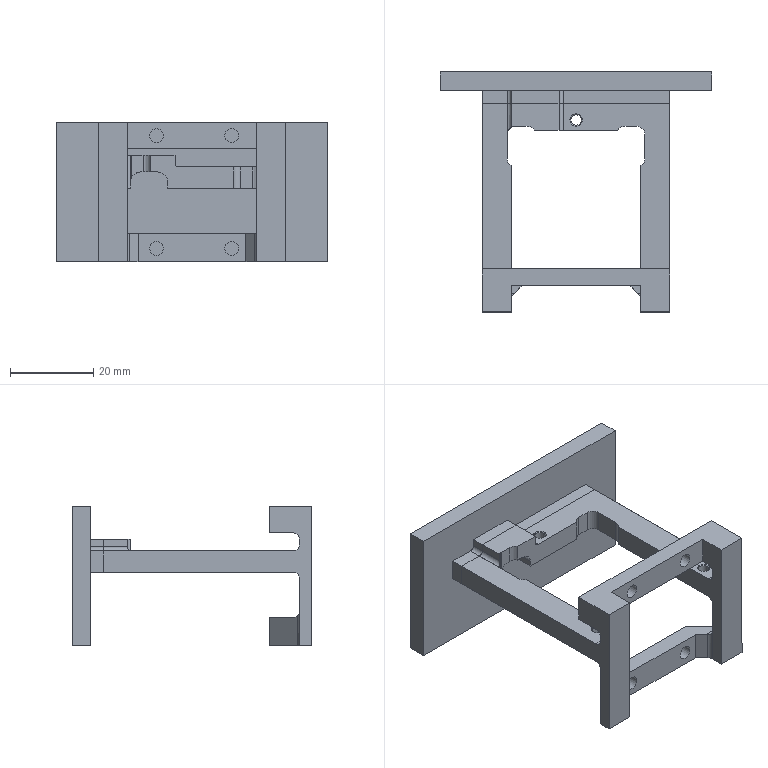CAM job | NX | 3+2 milling, drilling | part box 65 x 57.5 x 33.5 mm
Tools:
number,name,description,diameter,corner_radius,flute_length,length,flutes
7,D4R0.2,Milling Tool-5 Parameters,4.0,0.2,50.0,75.0,2
0,D2-6-D4-50-3T-FINISH,D2-6-D4-50-3T-精,2.0,0.0,6.0,7.0,3
5,D3-9-D4-50-3T-ROUGH,D3-9-D4-50-3T,3.0,0.0,9.0,10.0,3
6,D3-9-D4-50-3T-FINISH,D3-9-D4-50-3T-精,3.0,0.0,9.0,10.0,2
4,D4-12-D4-50-3T-FINISH,D4-12-D4-50-3T,4.0,0.0,12.0,50.0,3
2,D8-25-D8-60-3T-ROUGH,D8-25-D8-60-3T-粗,8.0,0.0,60.0,60.0,2
3,D8-25-D8-60-3T-FINISH,D8-25-D8-60-3T,8.0,0.0,25.0,60.0,3
1,D50面刀,D50面刀,50.0,0.0,30.0,30.0,4
0,点孔D3-50-90度,点孔D3-50-90度,3.0,0.0,0.0,50.0,2
10,钻头D2.5-35-61,钻刀D2.5-35-61,2.5,0.0,36.0,61.0,2
9,钻头D3.3-45-73,钻刀D3.3-45-73,3.3,0.0,45.0,73.0,2
11,上排M3-10-D4-52,上排M3-10-D4-52,3.0,0.0,10.0,12.0,2
8,倒角D4-90度,倒角D4-90度,4.0,0.0,5.0,50.0,2
Operations:
program,operation,operation_type,tool,method,geometry_group,spindle_rpm,surface_speed,feed_per_tooth,feed_cut,feed_plunge,cut_length_mm,path_length_mm,cut_time_min,machine_time_min
PROGRAM,动态粗_2_COPY,CavityMilling,D3-9-D4-50-3T-ROUGH,METHOD,WORKPIECE_55,6500.0,100.0,0.0769,1500.0,100.0,1748.83,3111.84,0.8121,0.9484
PROGRAM,动态粗_2,CavityMilling,D3-9-D4-50-3T-ROUGH,METHOD,WORKPIECE_55,6500.0,100.0,0.0769,1500.0,100.0,4077.343,4671.623,2.704,2.763
A1,PLANAR_MILL,PlanarMilling,D50面刀,METHOD,WORKPIECE_54,3500.0,549.0,0.0714,1000.0,100.0,109.0,165.0,0.109,0.1146
A2,动态粗,CavityMilling,D8-25-D8-60-3T-ROUGH,METHOD,WORKPIECE_54,6500.0,100.0,0.1178,3000.0,100.0,3498.632,4572.563,1.13,1.238
A3,PLANAR_MILL_2,PlanarMilling,D8-25-D8-60-3T-FINISH,METHOD,WORKPIECE_54,4500.0,113.0,0.0593,800.0,100.0,99.0,249,0.1238,0.1388
A3,PLANAR_MILL_1,PlanarMilling,D8-25-D8-60-3T-FINISH,METHOD,WORKPIECE_54,4500.0,113.0,0.0593,800.0,100.0,391.412,583.553,0.4893,0.5085
A3,PLANAR_MILL_3,PlanarMilling,D8-25-D8-60-3T-FINISH,METHOD,WORKPIECE_54,4500.0,113.0,0.0593,800.0,100.0,111.0,254.372,0.1388,0.1531
A3,PLANAR_MILL_4,PlanarMilling,D8-25-D8-60-3T-FINISH,METHOD,WORKPIECE_54,4500.0,113.0,0.0593,800.0,100.0,160.021,496.89,0.2,0.2337
A3,PLANAR_MILL_7,PlanarMilling,D8-25-D8-60-3T-FINISH,METHOD,WORKPIECE_54,4500.0,113.0,0.0593,800.0,100.0,84.618,178.618,0.1058,0.1152
A4,ZLEVEL_PROFILE_STEEP,ZLevelMilling,D4R0.2,METHOD,WORKPIECE_54,5500.0,69.0,0.1212,2000.0,100.0,1383.464,1535.341,0.6917,0.7069
A5,DRILLING,Operation,倒角D4-90度,METHOD,WORKPIECE_54,3000.0,37.0,0.0333,200.0,0.0,18.8,113.263,0.094,0.1034
A5,平面铣倒角,PlanarMilling,倒角D4-90度,METHOD,WORKPIECE_54,4500.0,56.0,0.1111,1000.0,100.0,201.133,299.185,0.2011,0.2109
A6,DRILLING_COPY,Operation,钻头D3.3-45-73,METHOD,WORKPIECE_54,3000.0,31.0,0.0333,200.0,0.0,36.0,147.663,0.18,0.1912
B1,动态粗_1,CavityMilling,D8-25-D8-60-3T-ROUGH,METHOD,WORKPIECE_55,6500.0,100.0,0.1178,3000.0,100.0,7238.783,8511.849,2.356,2.483
B1,DRILLING_1,Operation,点孔D3-50-90度,METHOD,WORKPIECE_55,2000.0,25.0,0.0375,150.0,0.0,12.0,163.129,0.08,0.0951
B1,DRILLING_1_COPY,Operation,钻头D2.5-35-61,METHOD,WORKPIECE_55,3000.0,23.0,0.025,150.0,0.0,33.0,205.129,0.22,0.2372
B1,DRILLING_1_COPY_COPY,Operation,上排M3-10-D4-52,METHOD,WORKPIECE_55,300.0,2.0,0.25,150.0,0.0,30.0,199.129,0.2,0.2169
B1,PLANAR_MILL_8_COPY_COPY_COPY_1,PlanarMilling,D3-9-D4-50-3T-ROUGH,METHOD,WORKPIECE_55,3000.0,28.0,0.25,1500.0,100.0,3326.577,4217.056,2.218,2.307
B1,PLANAR_MILL_8_COPY_1_COPY,PlanarMilling,D3-9-D4-50-3T-ROUGH,METHOD,WORKPIECE_55,3500.0,32.0,0.1429,1500.0,100.0,3153.789,4133.972,2.103,2.2
B1,PLANAR_MILL_8_COPY_2,PlanarMilling,D3-9-D4-50-3T-FINISH,METHOD,WORKPIECE_55,3000.0,28.0,0.1,600.0,100.0,175.515,999.904,0.2925,0.375
B1,PLANAR_MILL_5,PlanarMilling,D3-9-D4-50-3T-FINISH,METHOD,WORKPIECE_55,3000.0,42.0,0.0667,600.0,100.0,122.403,397.203,0.204,0.2315
B1,PLANAR_MILL_8_COPY_COPY_1,PlanarMilling,D3-9-D4-50-3T-FINISH,METHOD,WORKPIECE_55,3000.0,28.0,0.1,600.0,100.0,184.916,1005.127,0.3082,0.3902
B1,FLOOR_WALL_COPY_COPY,VolumeBased25DMillingOperation,D4-12-D4-50-3T-FINISH,METHOD,WORKPIECE_55,4000.0,50.0,0.05,600.0,100.0,291.788,428.588,0.4863,0.5
B1,FLOOR_WALL_COPY_COPY_COPY,VolumeBased25DMillingOperation,D4-12-D4-50-3T-FINISH,METHOD,WORKPIECE_55,4000.0,50.0,0.05,600.0,100.0,205.325,342.125,0.3422,0.3559
B1,FLOOR_WALL_1_COPY_1,VolumeBased25DMillingOperation,D8-25-D8-60-3T-ROUGH,METHOD,WORKPIECE_55,4000.0,50.0,0.05,600.0,100.0,144.983,258.983,0.2416,0.253
B1,FLOOR_WALL_1_COPY_COPY,VolumeBased25DMillingOperation,D8-25-D8-60-3T-ROUGH,METHOD,WORKPIECE_55,4000.0,50.0,0.05,600.0,100.0,144.983,258.983,0.2416,0.253
B1,动态粗_1_COPY,CavityMilling,D8-25-D8-60-3T-ROUGH,METHOD,WORKPIECE_55,6500.0,100.0,0.1178,3000.0,100.0,5894.717,6475.617,1.946,2.004
B1,PLANAR_MILL_8_COPY_1,PlanarMilling,D3-9-D4-50-3T-ROUGH,METHOD,WORKPIECE_55,3500.0,32.0,0.1429,1500.0,100.0,2428.779,3014.11,1.619,1.678
B1,PLANAR_MILL_8_COPY_COPY,PlanarMilling,D3-9-D4-50-3T-ROUGH,METHOD,WORKPIECE_55,3000.0,28.0,0.25,1500.0,100.0,2799.324,3221.226,1.866,1.908
B1,PLANAR_MILL_8,PlanarMilling,D3-9-D4-50-3T-FINISH,METHOD,WORKPIECE_55,3000.0,28.0,0.1,600.0,100.0,136.079,941.136,0.2268,0.3073
B1,PLANAR_MILL_8_COPY,PlanarMilling,D3-9-D4-50-3T-FINISH,METHOD,WORKPIECE_55,3000.0,28.0,0.1,600.0,100.0,155.413,952.913,0.259,0.3388
B1,FLOOR_WALL_1,VolumeBased25DMillingOperation,D4-12-D4-50-3T-FINISH,METHOD,WORKPIECE_55,4000.0,50.0,0.05,600.0,100.0,212.424,326.424,0.354,0.3654
B1,FLOOR_WALL_COPY,VolumeBased25DMillingOperation,D4-12-D4-50-3T-FINISH,METHOD,WORKPIECE_55,4000.0,50.0,0.05,600.0,100.0,425.045,702.747,0.7084,0.7362
B1,FLOOR_WALL_1_COPY,VolumeBased25DMillingOperation,D4-12-D4-50-3T-FINISH,METHOD,WORKPIECE_55,4000.0,50.0,0.05,600.0,100.0,215.003,329.003,0.3583,0.3697
B1,PLANAR_MILL_10,PlanarMilling,D8-25-D8-60-3T-ROUGH,METHOD,WORKPIECE_55,4000.0,50.0,0.05,600.0,100.0,201.0,649.646,0.335,0.3799
B1,动态粗_1_COPY_COPY,CavityMilling,D8-25-D8-60-3T-ROUGH,METHOD,WORKPIECE_55,6500.0,100.0,0.1178,3000.0,100.0,2076.441,2214.941,0.6921,0.706
B1,PLANAR_MILL_9,PlanarMilling,D4-12-D4-50-3T-FINISH,METHOD,WORKPIECE_55,4000.0,50.0,0.025,300.0,100.0,628.128,1662.21,2.094,2.197
B1,PLANAR_MILL_6,PlanarMilling,倒角D4-90度,METHOD,WORKPIECE_55,3500.0,43.0,0.1429,1000.0,100.0,125.699,223.699,0.1257,0.1355
B1,PLANAR_MILL_11,PlanarMilling,倒角D4-90度,METHOD,WORKPIECE_55,3500.0,43.0,0.1429,1000.0,100.0,184.852,302.852,0.1849,0.1967
B1,PLANAR_MILL_12,PlanarMilling,倒角D4-90度,METHOD,WORKPIECE_55,3500.0,43.0,0.1429,1000.0,100.0,53.0,151.0,0.053,0.0628
B1,PLANAR_MILL_11_COPY,PlanarMilling,倒角D4-90度,METHOD,WORKPIECE_55,3500.0,43.0,0.1429,1000.0,100.0,184.852,302.852,0.1849,0.1967
C1,PLANAR_PROFILING,PlanarMilling,D8-25-D8-60-3T-ROUGH,METHOD,C-G56,4500.0,113.0,0.1667,1500.0,100.0,966.0,1035.8,0.644,0.651
C2,PLANAR_PROFILING_COPY,PlanarMilling,D8-25-D8-60-3T-FINISH,METHOD,C-G56,4500.0,113.0,0.0741,1000.0,100.0,69.0,139.0,0.069,0.076
C3,PLANAR_PROFILING_1,PlanarMilling,D3-9-D4-50-3T-ROUGH,METHOD,C-G56,4500.0,42.0,0.1111,1500.0,100.0,857.733,925.733,0.5718,0.5786
C4,PLANAR_PROFILING_1_COPY,PlanarMilling,D3-9-D4-50-3T-ROUGH,METHOD,C-G56,4500.0,42.0,0.1111,1500.0,100.0,477.855,547.855,0.3186,0.3256
C5,PLANAR_PROFILING_1_COPY_1,PlanarMilling,D3-9-D4-50-3T-FINISH,METHOD,C-G56,4500.0,42.0,0.0889,800.0,100.0,35.712,103.712,0.0446,0.0514
C5,PLANAR_PROFILING_1_COPY_COPY,PlanarMilling,D3-9-D4-50-3T-FINISH,METHOD,C-G56,4500.0,42.0,0.0889,800.0,100.0,20.225,90.225,0.0253,0.0323
C6,平面铣倒角_1,PlanarMilling,倒角D4-90度,METHOD,C-G56,3500.0,43.0,0.1429,1000.0,100.0,124.163,180.163,0.1242,0.1298
C6,PLANAR_PROFILING_1_COPY_1_COPY,PlanarMilling,D2-6-D4-50-3T-FINISH,METHOD,C-G56,4500.0,42.0,0.0889,800.0,100.0,108.614,176.614,0.1358,0.1426